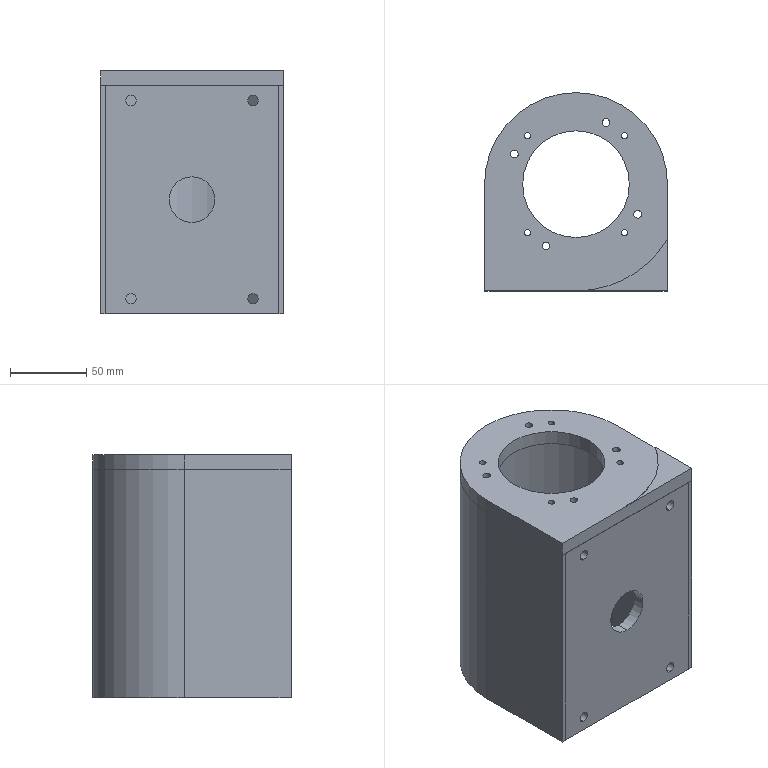Part | STEP file | Dual high-torque motor box SGN-4-01 | 3 solids | 56 faces | box 120 x 130 x 160 mm | volume 371672 mm3 | cylinder 32 | plane 24 | commonest cylinder face diameters 4.2 x8 5 x8 6.8 x8 30 x2 70 x2 120 x2